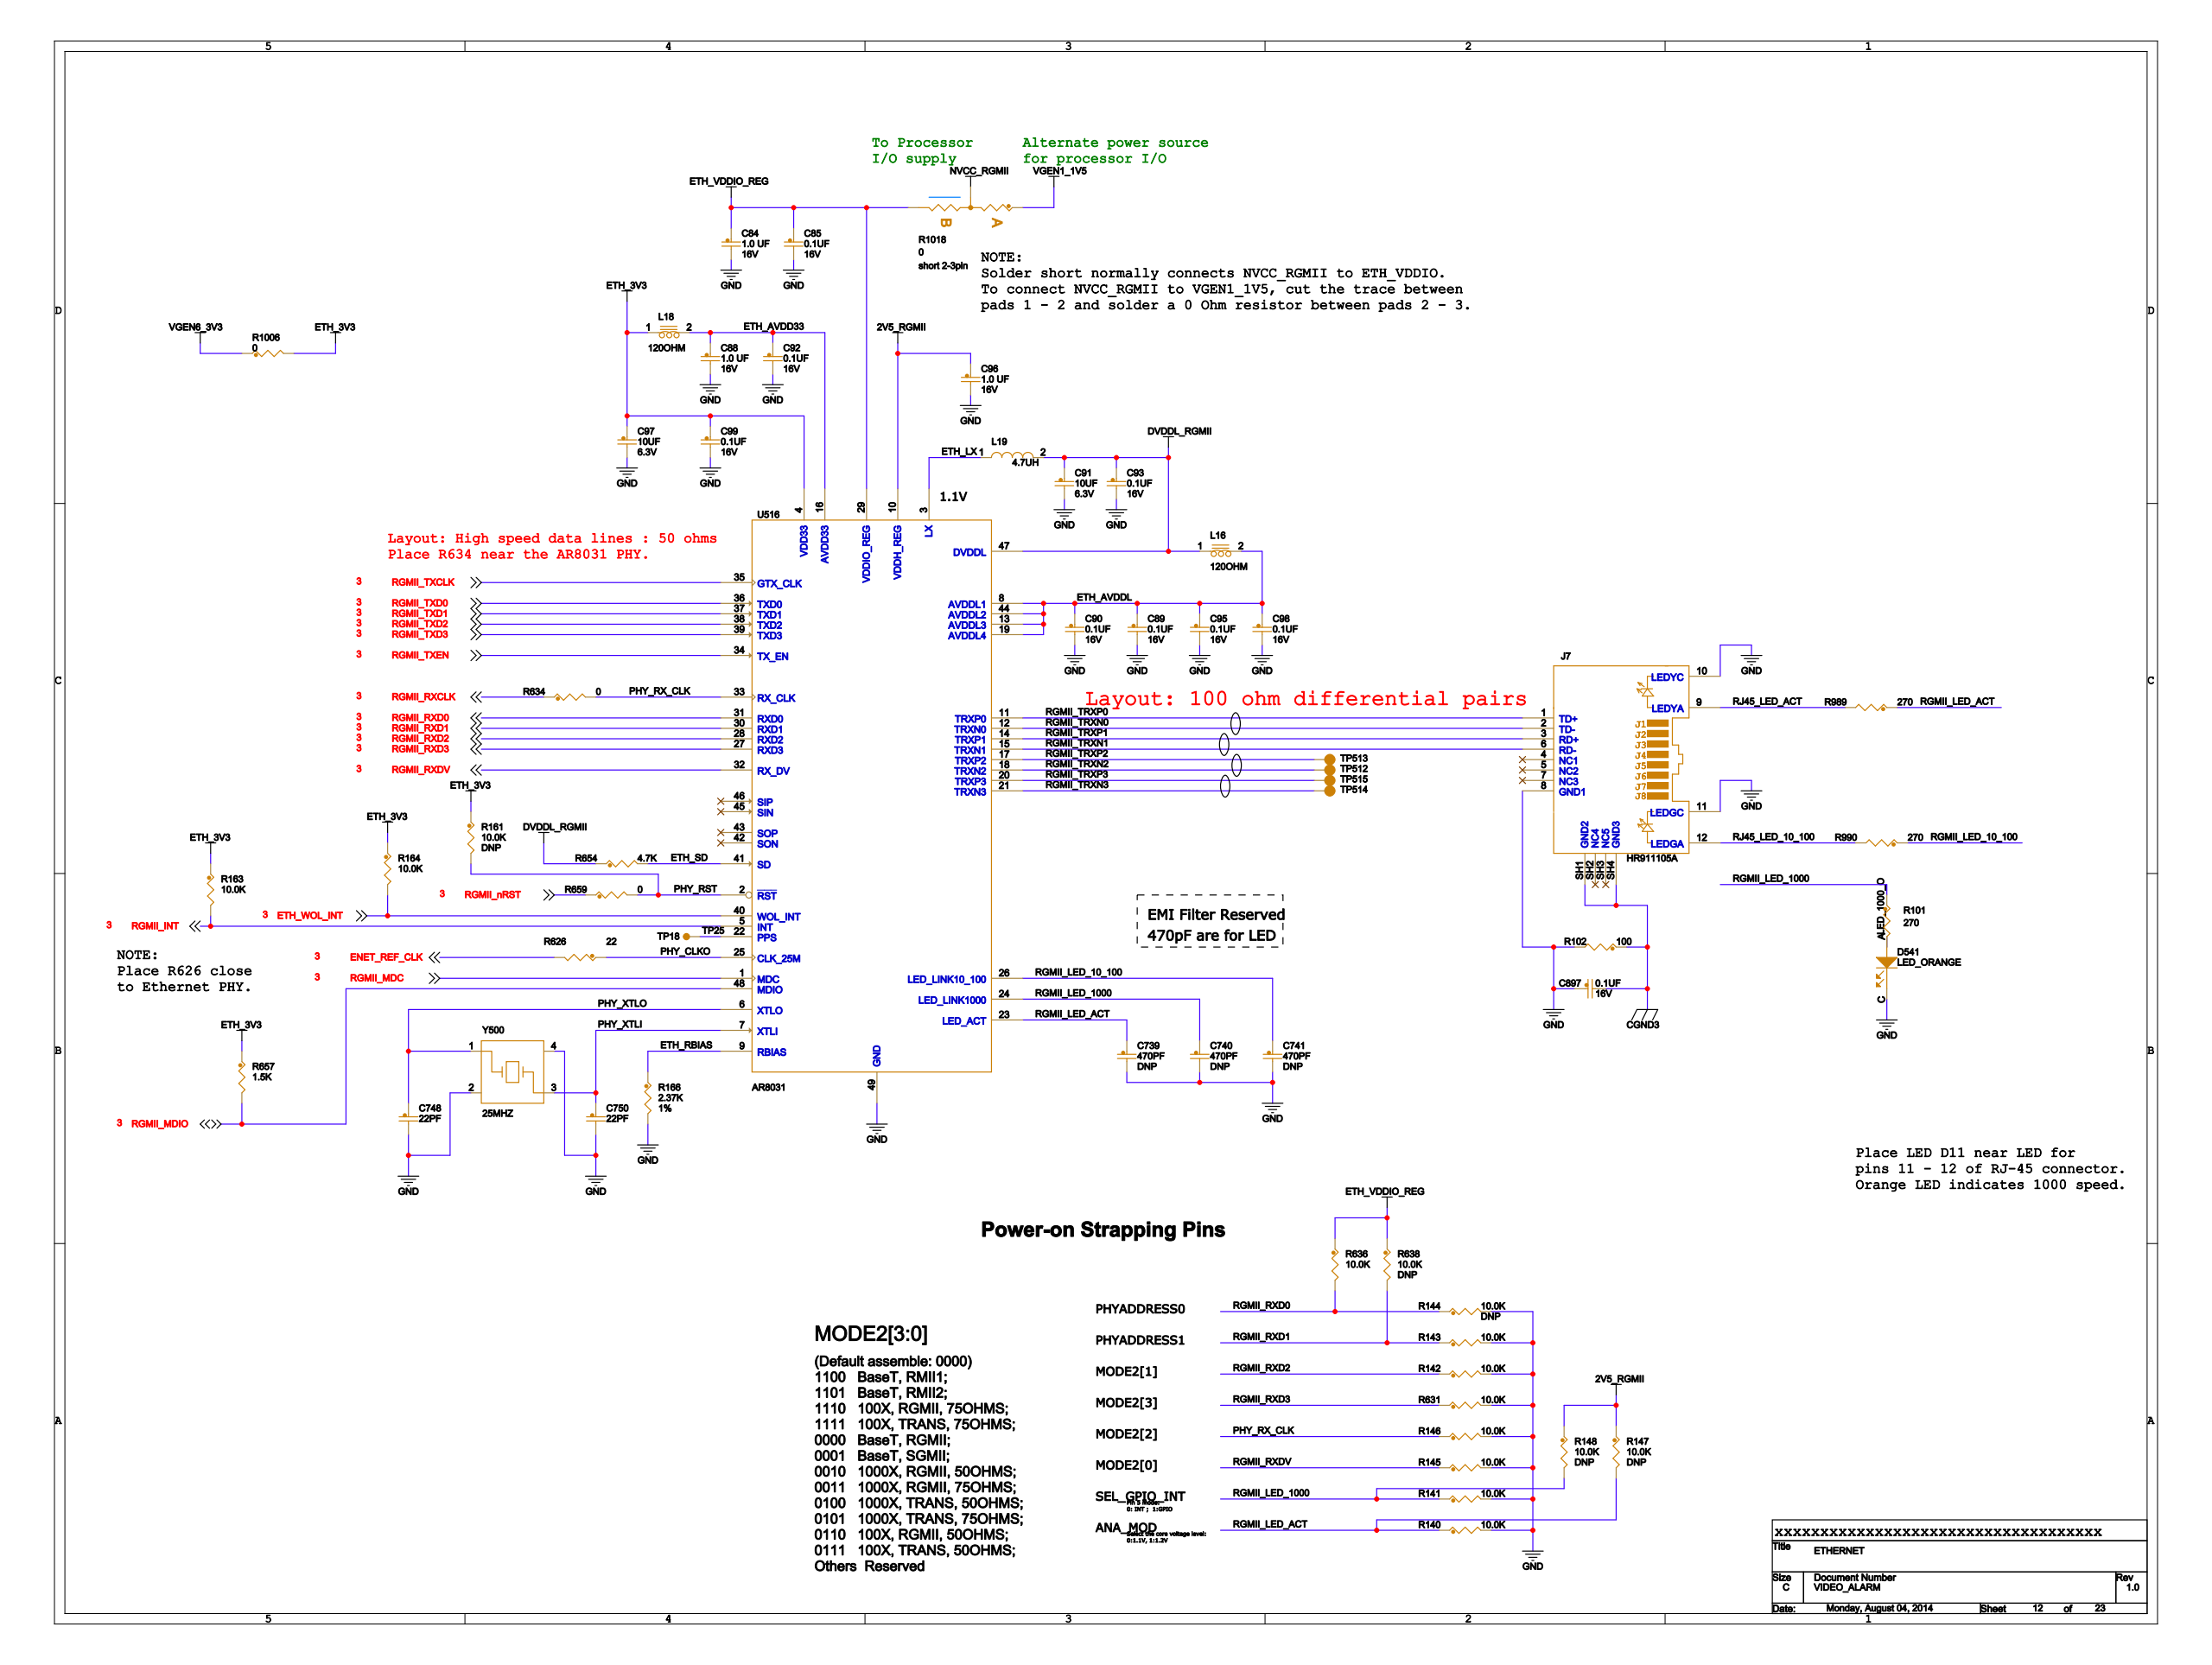Circuit board | Cadence Allegro | 994 parts | 728 nets | one sheet of the schematic
Parts on this sheet (reference | value | footprint):
C84 | 1.0 UF | 0603_CC
C85 | 0.1UF | 0603_CC
C88 | 1.0 UF | 0603_CC
C89 | 0.1UF | 0603_CC
C90 | 0.1UF | 0603_CC
C91 | 10UF | 0603_CC
C92 | 0.1UF | 0603_CC
C93 | 0.1UF | 0603_CC
C95 | 0.1UF | 0603_CC
C96 | 1.0 UF | 0603_CC
C97 | 10UF | 0603_CC
C98 | 0.1UF | 0603_CC
C99 | 0.1UF | 0603_CC
C739 | 470PF | 0603_CC
C740 | 470PF | 0603_CC
C741 | 470PF | 0603_CC
C748 | 22PF | 0603_CC
C750 | 22PF | 0603_CC
D541 | LED_ORANGE | LED_0603
J7 | HR911105A | HR911105A
J8 | 10029449-001RLF | HDMI
L16 | 120OHM | 0603_CC
L18 | 120OHM | 0603_CC
L19 | 4.7UH | IND_VLS3012_SM
R101 | 270 | 0603_CC
R102 | 100 | 0603_CC
R140 | 10.0K | 0603_CC
R141 | 10.0K | 0603_CC
R142 | 10.0K | 0603_CC
R143 | 10.0K | 0603_CC
R144 | 10.0K | 0603_CC
R145 | 10.0K | 0603_CC
R146 | 10.0K | 0603_CC
R147 | 10.0K | 0603_CC
R148 | 10.0K | 0603_CC
R161 | 10.0K | 0603_CC
R163 | 10.0K | 0603_CC
R164 | 10.0K | 0603_CC
R166 | 2.37K | 0603_CC
R626 | 22 | 0603_CC
R631 | 10.0K | 0603_CC
R634 | 0 | 0603_CC
R636 | 10.0K | 0603_CC
R638 | 10.0K | 0603_CC
R654 | 4.7K | 0603_CC
R657 | 1.5K | 0603_CC
R659 | 0 | 0603_CC
R989 | 270 | 0603_CC
R990 | 270 | 0603_CC
R1006 | 0 | 0603_CC
R1018 | 0 | R0805-X2
TP18 | TEST POINT | C035S
TP512 | TPAD_020 | TPAD_020
TP513 | TPAD_020 | TPAD_020
TP514 | TPAD_020 | TPAD_020
TP515 | TPAD_020 | TPAD_020
U516 | AR8031 | QFN48_0P4_6X6MM_EPAD
Y500 | 25MHZ | XTAL_4_7P2X5P2
Nets of these parts (net: part-pin ...):
GND: C84-2 C85-2 C88-2 C89-2 C90-2 C91-2 C92-2 C93-2 C95-2 C96-2 C97-2 C98-2 C99-2 C739-2 C740-2 C741-2 C748-2 C750-2 D541-C J7-8 J7-10 J7-11 R102-2 R140-2 R141-2 R142-2 R143-2 R144-2 R145-2 R146-2 R166-2 R631-2 Y500-2 Y500-4 J8-2 J8-5 J8-8 J8-11 U516-49
CGND3: J7-SH1 J7-SH4 R102-1
RJ45_LED_ACT: J7-9 R989-2
RGMII_TRXP0: J7-1 U516-11
RGMII_TRXP1: J7-3 U516-14
RGMII_TRXN0: J7-2 U516-12
RGMII_TRXN1: J7-6 U516-15
RJ45_LED_10_100: J7-12 R990-2
VGEN1_1V5: R1018-1
VGEN6_3V3: R1006-1
ETH_3V3: C97-1 C99-1 L18-1 R161-1 R163-1 R164-1 R657-1 R1006-2 U516-4
RGMII_MDIO: R657-2 U516-48
ETH_RBIAS: R166-1 U516-9
ETH_VDDIO_REG: C84-1 C85-1 R636-1 R638-1 R1018-3 U516-29
NVCC_RGMII: R1018-2
RGMII_LED_10_100: C741-1 R990-1 U516-26
RGMII_LED_ACT: C739-1 R140-1 R147-2 R989-1 U516-23
RGMII_LED_1000: C740-1 R101-1 R141-1 R148-2 U516-24
LED_1000_O: D541-A R101-2
RGMII_NRST: R659-1
PHY_RST: R161-2 R659-2 U516-2
RGMII_RXCLK: R634-1
PHY_RX_CLK: R146-1 R634-2 U516-33
RGMII_RXD1: R143-1 R638-2 U516-30
RGMII_RXD0: R144-1 R636-2 U516-31
RGMII_RXD3: R631-1 U516-27
ETH_WOL_INT: R164-2 U516-40
RGMII_INT: R163-2 U516-5
2V5_RGMII: C96-1 R147-1 R148-1 U516-10
RGMII_RXDV: R145-1 U516-32
RGMII_RXD2: R142-1 U516-28
PHY_XTLI: C750-1 Y500-3 U516-7
PHY_XTLO: C748-1 Y500-1 U516-6
ETH_AVDDL: C89-1 C90-1 C95-1 C98-1 L16-2 U516-8 U516-13 U516-19 U516-44
DVDDL_RGMII: C91-1 C93-1 L16-1 L19-2 R654-1 U516-47
ETH_AVDD33: C88-1 C92-1 L18-2 U516-16
PHY_CLKO: R626-1 U516-25
RGMII_TXCLK: U516-35
ETH_LX: L19-1 U516-3
RGMII_MDC: U516-1
TP25: TP18-1 U516-22
ETH_SD: R654-2 U516-41
RGMII_TRXN2: TP512-1 U516-18
RGMII_TRXN3: TP514-1 U516-21
RGMII_TRXP2: TP513-1 U516-17
RGMII_TRXP3: TP515-1 U516-20
RGMII_TXD0: U516-36
RGMII_TXD1: U516-37
RGMII_TXD2: U516-38
RGMII_TXD3: U516-39
RGMII_TXEN: U516-34
ENET_REF_CLK: R626-2